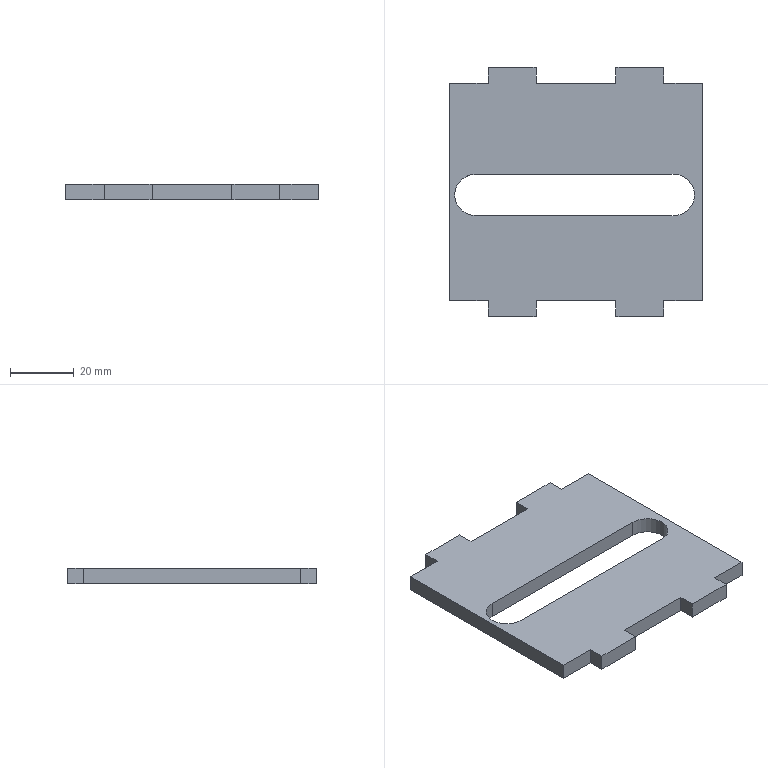Part | SolidWorks | features Extrusion 1, ICE 1 | 1 solid | 27 faces | box 79 x 77.9 x 5 mm | volume 23665 mm3 | plane 24 | cylinder 3 | commonest cylinder face diameters 12.879 x3
STEP:
#1=CARTESIAN_POINT('',(1.54,38.031,5.));
#2=VERTEX_POINT('',#1);
#3=CARTESIAN_POINT('',(7.98,44.471,5.));
#4=VERTEX_POINT('',#3);
#5=CARTESIAN_POINT('',(7.98,38.031,5.));
#6=DIRECTION('',(0.,0.,-1.));
#7=DIRECTION('',(-1.,0.,0.));
#8=AXIS2_PLACEMENT_3D('',#5,#6,#7);
#9=CIRCLE('',#8,6.44);
#10=EDGE_CURVE('',#2,#4,#9,.T.);
#11=ORIENTED_EDGE('',*,*,#10,.F.);
#12=CARTESIAN_POINT('',(1.54,38.031,0.));
#13=VERTEX_POINT('',#12);
#14=CARTESIAN_POINT('',(1.54,38.031,5.));
#15=DIRECTION('',(0.,0.,-1.));
#16=VECTOR('',#15,1000.);
#17=LINE('',#14,#16);
#18=EDGE_CURVE('',#2,#13,#17,.T.);
#19=ORIENTED_EDGE('',*,*,#18,.T.);
#20=CARTESIAN_POINT('',(7.98,44.471,0.));
#21=VERTEX_POINT('',#20);
#22=CARTESIAN_POINT('',(7.98,38.031,0.));
#23=DIRECTION('',(0.,0.,-1.));
#24=DIRECTION('',(-1.,0.,0.));
#25=AXIS2_PLACEMENT_3D('',#22,#23,#24);
#26=CIRCLE('',#25,6.44);
#27=EDGE_CURVE('',#13,#21,#26,.T.);
#28=ORIENTED_EDGE('',*,*,#27,.T.);
#29=CARTESIAN_POINT('',(7.98,44.471,5.));
#30=DIRECTION('',(0.,0.,-1.));
#31=VECTOR('',#30,1000.);
#32=LINE('',#29,#31);
#33=EDGE_CURVE('',#4,#21,#32,.T.);
#34=ORIENTED_EDGE('',*,*,#33,.F.);
#35=EDGE_LOOP('',(#11,#19,#28,#34));
#36=FACE_OUTER_BOUND('',#35,.T.);
#37=CARTESIAN_POINT('',(7.98,38.031,5.));
#38=DIRECTION('',(0.,0.,-1.));
#39=DIRECTION('',(-1.,0.,0.));
#40=AXIS2_PLACEMENT_3D('',#37,#38,#39);
#41=CYLINDRICAL_SURFACE('',#40,6.44);
#42=ADVANCED_FACE('',(#36),#41,.F.);
#43=CARTESIAN_POINT('',(52.,5.,0.));
#44=VERTEX_POINT('',#43);
#45=CARTESIAN_POINT('',(52.,0.,0.));
#46=VERTEX_POINT('',#45);
#47=CARTESIAN_POINT('',(52.,0.,0.));
#48=DIRECTION('',(0.,-1.,0.));
#49=VECTOR('',#48,1000.);
#50=LINE('',#47,#49);
#51=EDGE_CURVE('',#44,#46,#50,.T.);
#52=ORIENTED_EDGE('',*,*,#51,.T.);
#53=CARTESIAN_POINT('',(52.,0.,5.));
#54=VERTEX_POINT('',#53);
#55=CARTESIAN_POINT('',(52.,0.,5.));
#56=DIRECTION('',(0.,0.,-1.));
#57=VECTOR('',#56,1000.);
#58=LINE('',#55,#57);
#59=EDGE_CURVE('',#54,#46,#58,.T.);
#60=ORIENTED_EDGE('',*,*,#59,.F.);
#61=CARTESIAN_POINT('',(52.,5.,5.));
#62=VERTEX_POINT('',#61);
#63=CARTESIAN_POINT('',(52.,0.,5.));
#64=DIRECTION('',(0.,-1.,0.));
#65=VECTOR('',#64,1000.);
#66=LINE('',#63,#65);
#67=EDGE_CURVE('',#62,#54,#66,.T.);
#68=ORIENTED_EDGE('',*,*,#67,.F.);
#69=CARTESIAN_POINT('',(52.,5.,5.));
#70=DIRECTION('',(0.,0.,-1.));
#71=VECTOR('',#70,1000.);
#72=LINE('',#69,#71);
#73=EDGE_CURVE('',#62,#44,#72,.T.);
#74=ORIENTED_EDGE('',*,*,#73,.T.);
#75=EDGE_LOOP('',(#52,#60,#68,#74));
#76=FACE_OUTER_BOUND('',#75,.T.);
#77=CARTESIAN_POINT('',(52.,0.,5.));
#78=DIRECTION('',(1.,0.,0.));
#79=DIRECTION('',(0.,0.,-1.));
#80=AXIS2_PLACEMENT_3D('',#77,#78,#79);
#81=PLANE('',#80);
#82=ADVANCED_FACE('',(#76),#81,.F.);
#83=CARTESIAN_POINT('',(67.,0.,0.));
#84=VERTEX_POINT('',#83);
#85=CARTESIAN_POINT('',(52.,0.,0.));
#86=DIRECTION('',(1.,0.,0.));
#87=VECTOR('',#86,1000.);
#88=LINE('',#85,#87);
#89=EDGE_CURVE('',#46,#84,#88,.T.);
#90=ORIENTED_EDGE('',*,*,#89,.T.);
#91=CARTESIAN_POINT('',(67.,0.,5.));
#92=VERTEX_POINT('',#91);
#93=CARTESIAN_POINT('',(67.,0.,5.));
#94=DIRECTION('',(0.,0.,-1.));
#95=VECTOR('',#94,1000.);
#96=LINE('',#93,#95);
#97=EDGE_CURVE('',#92,#84,#96,.T.);
#98=ORIENTED_EDGE('',*,*,#97,.F.);
#99=CARTESIAN_POINT('',(52.,0.,5.));
#100=DIRECTION('',(1.,0.,0.));
#101=VECTOR('',#100,1000.);
#102=LINE('',#99,#101);
#103=EDGE_CURVE('',#54,#92,#102,.T.);
#104=ORIENTED_EDGE('',*,*,#103,.F.);
#105=ORIENTED_EDGE('',*,*,#59,.T.);
#106=EDGE_LOOP('',(#90,#98,#104,#105));
#107=FACE_OUTER_BOUND('',#106,.T.);
#108=CARTESIAN_POINT('',(52.,0.,5.));
#109=DIRECTION('',(0.,1.,0.));
#110=DIRECTION('',(-1.,0.,0.));
#111=AXIS2_PLACEMENT_3D('',#108,#109,#110);
#112=PLANE('',#111);
#113=ADVANCED_FACE('',(#107),#112,.F.);
#114=CARTESIAN_POINT('',(67.,5.,0.));
#115=VERTEX_POINT('',#114);
#116=CARTESIAN_POINT('',(67.,0.,0.));
#117=DIRECTION('',(0.,1.,0.));
#118=VECTOR('',#117,1000.);
#119=LINE('',#116,#118);
#120=EDGE_CURVE('',#84,#115,#119,.T.);
#121=ORIENTED_EDGE('',*,*,#120,.T.);
#122=CARTESIAN_POINT('',(67.,5.,5.));
#123=VERTEX_POINT('',#122);
#124=CARTESIAN_POINT('',(67.,5.,5.));
#125=DIRECTION('',(0.,0.,-1.));
#126=VECTOR('',#125,1000.);
#127=LINE('',#124,#126);
#128=EDGE_CURVE('',#123,#115,#127,.T.);
#129=ORIENTED_EDGE('',*,*,#128,.F.);
#130=CARTESIAN_POINT('',(67.,0.,5.));
#131=DIRECTION('',(0.,1.,0.));
#132=VECTOR('',#131,1000.);
#133=LINE('',#130,#132);
#134=EDGE_CURVE('',#92,#123,#133,.T.);
#135=ORIENTED_EDGE('',*,*,#134,.F.);
#136=ORIENTED_EDGE('',*,*,#97,.T.);
#137=EDGE_LOOP('',(#121,#129,#135,#136));
#138=FACE_OUTER_BOUND('',#137,.T.);
#139=CARTESIAN_POINT('',(67.,0.,5.));
#140=DIRECTION('',(-1.,0.,0.));
#141=DIRECTION('',(0.,0.,1.));
#142=AXIS2_PLACEMENT_3D('',#139,#140,#141);
#143=PLANE('',#142);
#144=ADVANCED_FACE('',(#138),#143,.F.);
#145=CARTESIAN_POINT('',(79.,5.,0.));
#146=VERTEX_POINT('',#145);
#147=CARTESIAN_POINT('',(67.,5.,0.));
#148=DIRECTION('',(1.,0.,0.));
#149=VECTOR('',#148,1000.);
#150=LINE('',#147,#149);
#151=EDGE_CURVE('',#115,#146,#150,.T.);
#152=ORIENTED_EDGE('',*,*,#151,.T.);
#153=CARTESIAN_POINT('',(79.,5.,5.));
#154=VERTEX_POINT('',#153);
#155=CARTESIAN_POINT('',(79.,5.,5.));
#156=DIRECTION('',(0.,0.,-1.));
#157=VECTOR('',#156,1000.);
#158=LINE('',#155,#157);
#159=EDGE_CURVE('',#154,#146,#158,.T.);
#160=ORIENTED_EDGE('',*,*,#159,.F.);
#161=CARTESIAN_POINT('',(67.,5.,5.));
#162=DIRECTION('',(1.,0.,0.));
#163=VECTOR('',#162,1000.);
#164=LINE('',#161,#163);
#165=EDGE_CURVE('',#123,#154,#164,.T.);
#166=ORIENTED_EDGE('',*,*,#165,.F.);
#167=ORIENTED_EDGE('',*,*,#128,.T.);
#168=EDGE_LOOP('',(#152,#160,#166,#167));
#169=FACE_OUTER_BOUND('',#168,.T.);
#170=CARTESIAN_POINT('',(67.,5.,5.));
#171=DIRECTION('',(0.,1.,0.));
#172=DIRECTION('',(-1.,0.,0.));
#173=AXIS2_PLACEMENT_3D('',#170,#171,#172);
#174=PLANE('',#173);
#175=ADVANCED_FACE('',(#169),#174,.F.);
#176=CARTESIAN_POINT('',(79.,72.9,0.));
#177=VERTEX_POINT('',#176);
#178=CARTESIAN_POINT('',(79.,5.,0.));
#179=DIRECTION('',(0.,1.,0.));
#180=VECTOR('',#179,1000.);
#181=LINE('',#178,#180);
#182=EDGE_CURVE('',#146,#177,#181,.T.);
#183=ORIENTED_EDGE('',*,*,#182,.T.);
#184=CARTESIAN_POINT('',(79.,72.9,5.));
#185=VERTEX_POINT('',#184);
#186=CARTESIAN_POINT('',(79.,72.9,5.));
#187=DIRECTION('',(0.,0.,-1.));
#188=VECTOR('',#187,1000.);
#189=LINE('',#186,#188);
#190=EDGE_CURVE('',#185,#177,#189,.T.);
#191=ORIENTED_EDGE('',*,*,#190,.F.);
#192=CARTESIAN_POINT('',(79.,5.,5.));
#193=DIRECTION('',(0.,1.,0.));
#194=VECTOR('',#193,1000.);
#195=LINE('',#192,#194);
#196=EDGE_CURVE('',#154,#185,#195,.T.);
#197=ORIENTED_EDGE('',*,*,#196,.F.);
#198=ORIENTED_EDGE('',*,*,#159,.T.);
#199=EDGE_LOOP('',(#183,#191,#197,#198));
#200=FACE_OUTER_BOUND('',#199,.T.);
#201=CARTESIAN_POINT('',(79.,5.,5.));
#202=DIRECTION('',(-1.,0.,0.));
#203=DIRECTION('',(0.,0.,1.));
#204=AXIS2_PLACEMENT_3D('',#201,#202,#203);
#205=PLANE('',#204);
#206=ADVANCED_FACE('',(#200),#205,.F.);
#207=CARTESIAN_POINT('',(67.,72.9,0.));
#208=VERTEX_POINT('',#207);
#209=CARTESIAN_POINT('',(79.,72.9,0.));
#210=DIRECTION('',(-1.,0.,0.));
#211=VECTOR('',#210,1000.);
#212=LINE('',#209,#211);
#213=EDGE_CURVE('',#177,#208,#212,.T.);
#214=ORIENTED_EDGE('',*,*,#213,.T.);
#215=CARTESIAN_POINT('',(67.,72.9,5.));
#216=VERTEX_POINT('',#215);
#217=CARTESIAN_POINT('',(67.,72.9,5.));
#218=DIRECTION('',(0.,0.,-1.));
#219=VECTOR('',#218,1000.);
#220=LINE('',#217,#219);
#221=EDGE_CURVE('',#216,#208,#220,.T.);
#222=ORIENTED_EDGE('',*,*,#221,.F.);
#223=CARTESIAN_POINT('',(79.,72.9,5.));
#224=DIRECTION('',(-1.,0.,0.));
#225=VECTOR('',#224,1000.);
#226=LINE('',#223,#225);
#227=EDGE_CURVE('',#185,#216,#226,.T.);
#228=ORIENTED_EDGE('',*,*,#227,.F.);
#229=ORIENTED_EDGE('',*,*,#190,.T.);
#230=EDGE_LOOP('',(#214,#222,#228,#229));
#231=FACE_OUTER_BOUND('',#230,.T.);
#232=CARTESIAN_POINT('',(79.,72.9,5.));
#233=DIRECTION('',(0.,-1.,0.));
#234=DIRECTION('',(0.,0.,-1.));
#235=AXIS2_PLACEMENT_3D('',#232,#233,#234);
#236=PLANE('',#235);
#237=ADVANCED_FACE('',(#231),#236,.F.);
#238=CARTESIAN_POINT('',(67.,77.9,0.));
#239=VERTEX_POINT('',#238);
#240=CARTESIAN_POINT('',(67.,77.9,0.));
#241=DIRECTION('',(0.,1.,0.));
#242=VECTOR('',#241,1000.);
#243=LINE('',#240,#242);
#244=EDGE_CURVE('',#208,#239,#243,.T.);
#245=ORIENTED_EDGE('',*,*,#244,.T.);
#246=CARTESIAN_POINT('',(67.,77.9,5.));
#247=VERTEX_POINT('',#246);
#248=CARTESIAN_POINT('',(67.,77.9,5.));
#249=DIRECTION('',(0.,0.,-1.));
#250=VECTOR('',#249,1000.);
#251=LINE('',#248,#250);
#252=EDGE_CURVE('',#247,#239,#251,.T.);
#253=ORIENTED_EDGE('',*,*,#252,.F.);
#254=CARTESIAN_POINT('',(67.,77.9,5.));
#255=DIRECTION('',(0.,1.,0.));
#256=VECTOR('',#255,1000.);
#257=LINE('',#254,#256);
#258=EDGE_CURVE('',#216,#247,#257,.T.);
#259=ORIENTED_EDGE('',*,*,#258,.F.);
#260=ORIENTED_EDGE('',*,*,#221,.T.);
#261=EDGE_LOOP('',(#245,#253,#259,#260));
#262=FACE_OUTER_BOUND('',#261,.T.);
#263=CARTESIAN_POINT('',(67.,77.9,5.));
#264=DIRECTION('',(-1.,0.,0.));
#265=DIRECTION('',(0.,0.,1.));
#266=AXIS2_PLACEMENT_3D('',#263,#264,#265);
#267=PLANE('',#266);
#268=ADVANCED_FACE('',(#262),#267,.F.);
#269=CARTESIAN_POINT('',(52.,77.9,0.));
#270=VERTEX_POINT('',#269);
#271=CARTESIAN_POINT('',(52.,77.9,0.));
#272=DIRECTION('',(-1.,0.,0.));
#273=VECTOR('',#272,1000.);
#274=LINE('',#271,#273);
#275=EDGE_CURVE('',#239,#270,#274,.T.);
#276=ORIENTED_EDGE('',*,*,#275,.T.);
#277=CARTESIAN_POINT('',(52.,77.9,5.));
#278=VERTEX_POINT('',#277);
#279=CARTESIAN_POINT('',(52.,77.9,5.));
#280=DIRECTION('',(0.,0.,-1.));
#281=VECTOR('',#280,1000.);
#282=LINE('',#279,#281);
#283=EDGE_CURVE('',#278,#270,#282,.T.);
#284=ORIENTED_EDGE('',*,*,#283,.F.);
#285=CARTESIAN_POINT('',(52.,77.9,5.));
#286=DIRECTION('',(-1.,0.,0.));
#287=VECTOR('',#286,1000.);
#288=LINE('',#285,#287);
#289=EDGE_CURVE('',#247,#278,#288,.T.);
#290=ORIENTED_EDGE('',*,*,#289,.F.);
#291=ORIENTED_EDGE('',*,*,#252,.T.);
#292=EDGE_LOOP('',(#276,#284,#290,#291));
#293=FACE_OUTER_BOUND('',#292,.T.);
#294=CARTESIAN_POINT('',(52.,77.9,5.));
#295=DIRECTION('',(0.,-1.,0.));
#296=DIRECTION('',(0.,0.,-1.));
#297=AXIS2_PLACEMENT_3D('',#294,#295,#296);
#298=PLANE('',#297);
#299=ADVANCED_FACE('',(#293),#298,.F.);
#300=CARTESIAN_POINT('',(52.,72.9,0.));
#301=VERTEX_POINT('',#300);
#302=CARTESIAN_POINT('',(52.,77.9,0.));
#303=DIRECTION('',(0.,-1.,0.));
#304=VECTOR('',#303,1000.);
#305=LINE('',#302,#304);
#306=EDGE_CURVE('',#270,#301,#305,.T.);
#307=ORIENTED_EDGE('',*,*,#306,.T.);
#308=CARTESIAN_POINT('',(52.,72.9,5.));
#309=VERTEX_POINT('',#308);
#310=CARTESIAN_POINT('',(52.,72.9,5.));
#311=DIRECTION('',(0.,0.,-1.));
#312=VECTOR('',#311,1000.);
#313=LINE('',#310,#312);
#314=EDGE_CURVE('',#309,#301,#313,.T.);
#315=ORIENTED_EDGE('',*,*,#314,.F.);
#316=CARTESIAN_POINT('',(52.,77.9,5.));
#317=DIRECTION('',(0.,-1.,0.));
#318=VECTOR('',#317,1000.);
#319=LINE('',#316,#318);
#320=EDGE_CURVE('',#278,#309,#319,.T.);
#321=ORIENTED_EDGE('',*,*,#320,.F.);
#322=ORIENTED_EDGE('',*,*,#283,.T.);
#323=EDGE_LOOP('',(#307,#315,#321,#322));
#324=FACE_OUTER_BOUND('',#323,.T.);
#325=CARTESIAN_POINT('',(52.,77.9,5.));
#326=DIRECTION('',(1.,0.,0.));
#327=DIRECTION('',(0.,1.,0.));
#328=AXIS2_PLACEMENT_3D('',#325,#326,#327);
#329=PLANE('',#328);
#330=ADVANCED_FACE('',(#324),#329,.F.);
#331=CARTESIAN_POINT('',(27.,72.9,0.));
#332=VERTEX_POINT('',#331);
#333=CARTESIAN_POINT('',(52.,72.9,0.));
#334=DIRECTION('',(-1.,0.,0.));
#335=VECTOR('',#334,1000.);
#336=LINE('',#333,#335);
#337=EDGE_CURVE('',#301,#332,#336,.T.);
#338=ORIENTED_EDGE('',*,*,#337,.T.);
#339=CARTESIAN_POINT('',(27.,72.9,5.));
#340=VERTEX_POINT('',#339);
#341=CARTESIAN_POINT('',(27.,72.9,5.));
#342=DIRECTION('',(0.,0.,-1.));
#343=VECTOR('',#342,1000.);
#344=LINE('',#341,#343);
#345=EDGE_CURVE('',#340,#332,#344,.T.);
#346=ORIENTED_EDGE('',*,*,#345,.F.);
#347=CARTESIAN_POINT('',(52.,72.9,5.));
#348=DIRECTION('',(-1.,0.,0.));
#349=VECTOR('',#348,1000.);
#350=LINE('',#347,#349);
#351=EDGE_CURVE('',#309,#340,#350,.T.);
#352=ORIENTED_EDGE('',*,*,#351,.F.);
#353=ORIENTED_EDGE('',*,*,#314,.T.);
#354=EDGE_LOOP('',(#338,#346,#352,#353));
#355=FACE_OUTER_BOUND('',#354,.T.);
#356=CARTESIAN_POINT('',(52.,72.9,5.));
#357=DIRECTION('',(0.,-1.,0.));
#358=DIRECTION('',(0.,0.,-1.));
#359=AXIS2_PLACEMENT_3D('',#356,#357,#358);
#360=PLANE('',#359);
#361=ADVANCED_FACE('',(#355),#360,.F.);
#362=CARTESIAN_POINT('',(27.,77.9,0.));
#363=VERTEX_POINT('',#362);
#364=CARTESIAN_POINT('',(27.,77.9,0.));
#365=DIRECTION('',(0.,1.,0.));
#366=VECTOR('',#365,1000.);
#367=LINE('',#364,#366);
#368=EDGE_CURVE('',#332,#363,#367,.T.);
#369=ORIENTED_EDGE('',*,*,#368,.T.);
#370=CARTESIAN_POINT('',(27.,77.9,5.));
#371=VERTEX_POINT('',#370);
#372=CARTESIAN_POINT('',(27.,77.9,5.));
#373=DIRECTION('',(0.,0.,-1.));
#374=VECTOR('',#373,1000.);
#375=LINE('',#372,#374);
#376=EDGE_CURVE('',#371,#363,#375,.T.);
#377=ORIENTED_EDGE('',*,*,#376,.F.);
#378=CARTESIAN_POINT('',(27.,77.9,5.));
#379=DIRECTION('',(0.,1.,0.));
#380=VECTOR('',#379,1000.);
#381=LINE('',#378,#380);
#382=EDGE_CURVE('',#340,#371,#381,.T.);
#383=ORIENTED_EDGE('',*,*,#382,.F.);
#384=ORIENTED_EDGE('',*,*,#345,.T.);
#385=EDGE_LOOP('',(#369,#377,#383,#384));
#386=FACE_OUTER_BOUND('',#385,.T.);
#387=CARTESIAN_POINT('',(27.,77.9,5.));
#388=DIRECTION('',(-1.,0.,0.));
#389=DIRECTION('',(0.,-1.,0.));
#390=AXIS2_PLACEMENT_3D('',#387,#388,#389);
#391=PLANE('',#390);
#392=ADVANCED_FACE('',(#386),#391,.F.);
#393=CARTESIAN_POINT('',(12.,77.9,0.));
#394=VERTEX_POINT('',#393);
#395=CARTESIAN_POINT('',(12.,77.9,0.));
#396=DIRECTION('',(-1.,0.,0.));
#397=VECTOR('',#396,1000.);
#398=LINE('',#395,#397);
#399=EDGE_CURVE('',#363,#394,#398,.T.);
#400=ORIENTED_EDGE('',*,*,#399,.T.);
#401=CARTESIAN_POINT('',(12.,77.9,5.));
#402=VERTEX_POINT('',#401);
#403=CARTESIAN_POINT('',(12.,77.9,5.));
#404=DIRECTION('',(0.,0.,-1.));
#405=VECTOR('',#404,1000.);
#406=LINE('',#403,#405);
#407=EDGE_CURVE('',#402,#394,#406,.T.);
#408=ORIENTED_EDGE('',*,*,#407,.F.);
#409=CARTESIAN_POINT('',(12.,77.9,5.));
#410=DIRECTION('',(-1.,0.,0.));
#411=VECTOR('',#410,1000.);
#412=LINE('',#409,#411);
#413=EDGE_CURVE('',#371,#402,#412,.T.);
#414=ORIENTED_EDGE('',*,*,#413,.F.);
#415=ORIENTED_EDGE('',*,*,#376,.T.);
#416=EDGE_LOOP('',(#400,#408,#414,#415));
#417=FACE_OUTER_BOUND('',#416,.T.);
#418=CARTESIAN_POINT('',(12.,77.9,5.));
#419=DIRECTION('',(0.,-1.,0.));
#420=DIRECTION('',(0.,0.,-1.));
#421=AXIS2_PLACEMENT_3D('',#418,#419,#420);
#422=PLANE('',#421);
#423=ADVANCED_FACE('',(#417),#422,.F.);
#424=CARTESIAN_POINT('',(12.,72.9,0.));
#425=VERTEX_POINT('',#424);
#426=CARTESIAN_POINT('',(12.,77.9,0.));
#427=DIRECTION('',(0.,-1.,0.));
#428=VECTOR('',#427,1000.);
#429=LINE('',#426,#428);
#430=EDGE_CURVE('',#394,#425,#429,.T.);
#431=ORIENTED_EDGE('',*,*,#430,.T.);
#432=CARTESIAN_POINT('',(12.,72.9,5.));
#433=VERTEX_POINT('',#432);
#434=CARTESIAN_POINT('',(12.,72.9,5.));
#435=DIRECTION('',(0.,0.,-1.));
#436=VECTOR('',#435,1000.);
#437=LINE('',#434,#436);
#438=EDGE_CURVE('',#433,#425,#437,.T.);
#439=ORIENTED_EDGE('',*,*,#438,.F.);
#440=CARTESIAN_POINT('',(12.,77.9,5.));
#441=DIRECTION('',(0.,-1.,0.));
#442=VECTOR('',#441,1000.);
#443=LINE('',#440,#442);
#444=EDGE_CURVE('',#402,#433,#443,.T.);
#445=ORIENTED_EDGE('',*,*,#444,.F.);
#446=ORIENTED_EDGE('',*,*,#407,.T.);
#447=EDGE_LOOP('',(#431,#439,#445,#446));
#448=FACE_OUTER_BOUND('',#447,.T.);
#449=CARTESIAN_POINT('',(12.,77.9,5.));
#450=DIRECTION('',(1.,0.,0.));
#451=DIRECTION('',(0.,0.,-1.));
#452=AXIS2_PLACEMENT_3D('',#449,#450,#451);
#453=PLANE('',#452);
#454=ADVANCED_FACE('',(#448),#453,.F.);
#455=CARTESIAN_POINT('',(0.,72.9,0.));
#456=VERTEX_POINT('',#455);
#457=CARTESIAN_POINT('',(12.,72.9,0.));
#458=DIRECTION('',(-1.,0.,0.));
#459=VECTOR('',#458,1000.);
#460=LINE('',#457,#459);
#461=EDGE_CURVE('',#425,#456,#460,.T.);
#462=ORIENTED_EDGE('',*,*,#461,.T.);
#463=CARTESIAN_POINT('',(0.,72.9,5.));
#464=VERTEX_POINT('',#463);
#465=CARTESIAN_POINT('',(0.,72.9,5.));
#466=DIRECTION('',(0.,0.,-1.));
#467=VECTOR('',#466,1000.);
#468=LINE('',#465,#467);
#469=EDGE_CURVE('',#464,#456,#468,.T.);
#470=ORIENTED_EDGE('',*,*,#469,.F.);
#471=CARTESIAN_POINT('',(12.,72.9,5.));
#472=DIRECTION('',(-1.,0.,0.));
#473=VECTOR('',#472,1000.);
#474=LINE('',#471,#473);
#475=EDGE_CURVE('',#433,#464,#474,.T.);
#476=ORIENTED_EDGE('',*,*,#475,.F.);
#477=ORIENTED_EDGE('',*,*,#438,.T.);
#478=EDGE_LOOP('',(#462,#470,#476,#477));
#479=FACE_OUTER_BOUND('',#478,.T.);
#480=CARTESIAN_POINT('',(12.,72.9,5.));
#481=DIRECTION('',(0.,-1.,0.));
#482=DIRECTION('',(0.,0.,-1.));
#483=AXIS2_PLACEMENT_3D('',#480,#481,#482);
#484=PLANE('',#483);
#485=ADVANCED_FACE('',(#479),#484,.F.);
#486=CARTESIAN_POINT('',(0.,5.,0.));
#487=VERTEX_POINT('',#486);
#488=CARTESIAN_POINT('',(0.,5.,0.));
#489=DIRECTION('',(0.,-1.,0.));
#490=VECTOR('',#489,1000.);
#491=LINE('',#488,#490);
#492=EDGE_CURVE('',#456,#487,#491,.T.);
#493=ORIENTED_EDGE('',*,*,#492,.T.);
#494=CARTESIAN_POINT('',(0.,5.,5.));
#495=VERTEX_POINT('',#494);
#496=CARTESIAN_POINT('',(0.,5.,5.));
#497=DIRECTION('',(0.,0.,-1.));
#498=VECTOR('',#497,1000.);
#499=LINE('',#496,#498);
#500=EDGE_CURVE('',#495,#487,#499,.T.);
#501=ORIENTED_EDGE('',*,*,#500,.F.);
#502=CARTESIAN_POINT('',(0.,5.,5.));
#503=DIRECTION('',(0.,-1.,0.));
#504=VECTOR('',#503,1000.);
#505=LINE('',#502,#504);
#506=EDGE_CURVE('',#464,#495,#505,.T.);
#507=ORIENTED_EDGE('',*,*,#506,.F.);
#508=ORIENTED_EDGE('',*,*,#469,.T.);
#509=EDGE_LOOP('',(#493,#501,#507,#508));
#510=FACE_OUTER_BOUND('',#509,.T.);
#511=CARTESIAN_POINT('',(0.,5.,5.));
#512=DIRECTION('',(1.,0.,0.));
#513=DIRECTION('',(0.,1.,0.));
#514=AXIS2_PLACEMENT_3D('',#511,#512,#513);
#515=PLANE('',#514);
#516=ADVANCED_FACE('',(#510),#515,.F.);
#517=CARTESIAN_POINT('',(12.,5.,0.));
#518=VERTEX_POINT('',#517);
#519=CARTESIAN_POINT('',(0.,5.,0.));
#520=DIRECTION('',(1.,0.,0.));
#521=VECTOR('',#520,1000.);
#522=LINE('',#519,#521);
#523=EDGE_CURVE('',#487,#518,#522,.T.);
#524=ORIENTED_EDGE('',*,*,#523,.T.);
#525=CARTESIAN_POINT('',(12.,5.,5.));
#526=VERTEX_POINT('',#525);
#527=CARTESIAN_POINT('',(12.,5.,5.));
#528=DIRECTION('',(0.,0.,-1.));
#529=VECTOR('',#528,1000.);
#530=LINE('',#527,#529);
#531=EDGE_CURVE('',#526,#518,#530,.T.);
#532=ORIENTED_EDGE('',*,*,#531,.F.);
#533=CARTESIAN_POINT('',(0.,5.,5.));
#534=DIRECTION('',(1.,0.,0.));
#535=VECTOR('',#534,1000.);
#536=LINE('',#533,#535);
#537=EDGE_CURVE('',#495,#526,#536,.T.);
#538=ORIENTED_EDGE('',*,*,#537,.F.);
#539=ORIENTED_EDGE('',*,*,#500,.T.);
#540=EDGE_LOOP('',(#524,#532,#538,#539));
#541=FACE_OUTER_BOUND('',#540,.T.);
#542=CARTESIAN_POINT('',(0.,5.,5.));
#543=DIRECTION('',(0.,1.,0.));
#544=DIRECTION('',(-1.,0.,0.));
#545=AXIS2_PLACEMENT_3D('',#542,#543,#544);
#546=PLANE('',#545);
#547=ADVANCED_FACE('',(#541),#546,.F.);
#548=CARTESIAN_POINT('',(12.,0.,0.));
#549=VERTEX_POINT('',#548);
#550=CARTESIAN_POINT('',(12.,0.,0.));
#551=DIRECTION('',(0.,-1.,0.));
#552=VECTOR('',#551,1000.);
#553=LINE('',#550,#552);
#554=EDGE_CURVE('',#518,#549,#553,.T.);
#555=ORIENTED_EDGE('',*,*,#554,.T.);
#556=CARTESIAN_POINT('',(12.,0.,5.));
#557=VERTEX_POINT('',#556);
#558=CARTESIAN_POINT('',(12.,0.,5.));
#559=DIRECTION('',(0.,0.,-1.));
#560=VECTOR('',#559,1000.);
#561=LINE('',#558,#560);
#562=EDGE_CURVE('',#557,#549,#561,.T.);
#563=ORIENTED_EDGE('',*,*,#562,.F.);
#564=CARTESIAN_POINT('',(12.,0.,5.));
#565=DIRECTION('',(0.,-1.,0.));
#566=VECTOR('',#565,1000.);
#567=LINE('',#564,#566);
#568=EDGE_CURVE('',#526,#557,#567,.T.);
#569=ORIENTED_EDGE('',*,*,#568,.F.);
#570=ORIENTED_EDGE('',*,*,#531,.T.);
#571=EDGE_LOOP('',(#555,#563,#569,#570));
#572=FACE_OUTER_BOUND('',#571,.T.);
#573=CARTESIAN_POINT('',(12.,0.,5.));
#574=DIRECTION('',(1.,0.,0.));
#575=DIRECTION('',(0.,0.,-1.));
#576=AXIS2_PLACEMENT_3D('',#573,#574,#575);
#577=PLANE('',#576);
#578=ADVANCED_FACE('',(#572),#577,.F.);
#579=CARTESIAN_POINT('',(27.,0.,0.));
#580=VERTEX_POINT('',#579);
#581=CARTESIAN_POINT('',(12.,0.,0.));
#582=DIRECTION('',(1.,0.,0.));
#583=VECTOR('',#582,1000.);
#584=LINE('',#581,#583);
#585=EDGE_CURVE('',#549,#580,#584,.T.);
#586=ORIENTED_EDGE('',*,*,#585,.T.);
#587=CARTESIAN_POINT('',(27.,0.,5.));
#588=VERTEX_POINT('',#587);
#589=CARTESIAN_POINT('',(27.,0.,5.));
#590=DIRECTION('',(0.,0.,-1.));
#591=VECTOR('',#590,1000.);
#592=LINE('',#589,#591);
#593=EDGE_CURVE('',#588,#580,#592,.T.);
#594=ORIENTED_EDGE('',*,*,#593,.F.);
#595=CARTESIAN_POINT('',(12.,0.,5.));
#596=DIRECTION('',(1.,0.,0.));
#597=VECTOR('',#596,1000.);
#598=LINE('',#595,#597);
#599=EDGE_CURVE('',#557,#588,#598,.T.);
#600=ORIENTED_EDGE('',*,*,#599,.F.);
#601=ORIENTED_EDGE('',*,*,#562,.T.);
#602=EDGE_LOOP('',(#586,#594,#600,#601));
#603=FACE_OUTER_BOUND('',#602,.T.);
#604=CARTESIAN_POINT('',(12.,0.,5.));
#605=DIRECTION('',(0.,1.,0.));
#606=DIRECTION('',(-1.,0.,0.));
#607=AXIS2_PLACEMENT_3D('',#604,#605,#606);
#608=PLANE('',#607);
#609=ADVANCED_FACE('',(#603),#608,.F.);
#610=CARTESIAN_POINT('',(27.,5.,0.));
#611=VERTEX_POINT('',#610);
#612=CARTESIAN_POINT('',(27.,0.,0.));
#613=DIRECTION('',(0.,1.,0.));
#614=VECTOR('',#613,1000.);
#615=LINE('',#612,#614);
#616=EDGE_CURVE('',#580,#611,#615,.T.);
#617=ORIENTED_EDGE('',*,*,#616,.T.);
#618=CARTESIAN_POINT('',(27.,5.,5.));
#619=VERTEX_POINT('',#618);
#620=CARTESIAN_POINT('',(27.,5.,5.));
#621=DIRECTION('',(0.,0.,-1.));
#622=VECTOR('',#621,1000.);
#623=LINE('',#620,#622);
#624=EDGE_CURVE('',#619,#611,#623,.T.);
#625=ORIENTED_EDGE('',*,*,#624,.F.);
#626=CARTESIAN_POINT('',(27.,0.,5.));
#627=DIRECTION('',(0.,1.,0.));
#628=VECTOR('',#627,1000.);
#629=LINE('',#626,#628);
#630=EDGE_CURVE('',#588,#619,#629,.T.);
#631=ORIENTED_EDGE('',*,*,#630,.F.);
#632=ORIENTED_EDGE('',*,*,#593,.T.);
#633=EDGE_LOOP('',(#617,#625,#631,#632));
#634=FACE_OUTER_BOUND('',#633,.T.);
#635=CARTESIAN_POINT('',(27.,0.,5.));
#636=DIRECTION('',(-1.,0.,0.));
#637=DIRECTION('',(0.,0.,1.));
#638=AXIS2_PLACEMENT_3D('',#635,#636,#637);
#639=PLANE('',#638);
#640=ADVANCED_FACE('',(#634),#639,.F.);
#641=CARTESIAN_POINT('',(27.,5.,0.));
#642=DIRECTION('',(1.,0.,0.));
#643=VECTOR('',#642,1000.);
#644=LINE('',#641,#643);
#645=EDGE_CURVE('',#611,#44,#644,.T.);
#646=ORIENTED_EDGE('',*,*,#645,.T.);
#647=ORIENTED_EDGE('',*,*,#73,.F.);
#648=CARTESIAN_POINT('',(27.,5.,5.));
#649=DIRECTION('',(1.,0.,0.));
#650=VECTOR('',#649,1000.);
#651=LINE('',#648,#650);
#652=EDGE_CURVE('',#619,#62,#651,.T.);
#653=ORIENTED_EDGE('',*,*,#652,.F.);
#654=ORIENTED_EDGE('',*,*,#624,.T.);
#655=EDGE_LOOP('',(#646,#647,#653,#654));
#656=FACE_OUTER_BOUND('',#655,.T.);
#657=CARTESIAN_POINT('',(27.,5.,5.));
#658=DIRECTION('',(0.,1.,0.));
#659=DIRECTION('',(0.,0.,1.));
#660=AXIS2_PLACEMENT_3D('',#657,#658,#659);
#661=PLANE('',#660);
#662=ADVANCED_FACE('',(#656),#661,.F.);
#663=CARTESIAN_POINT('',(70.163,44.471,5.));
#664=VERTEX_POINT('',#663);
#665=CARTESIAN_POINT('',(70.163,44.471,5.));
#666=DIRECTION('',(1.,0.,0.));
#667=VECTOR('',#666,1000.);
#668=LINE('',#665,#667);
#669=EDGE_CURVE('',#4,#664,#668,.T.);
#670=ORIENTED_EDGE('',*,*,#669,.T.);
#671=CARTESIAN_POINT('',(70.163,31.592,5.));
#672=VERTEX_POINT('',#671);
#673=CARTESIAN_POINT('',(70.163,38.031,5.));
#674=DIRECTION('',(0.,0.,-1.));
#675=DIRECTION('',(-1.,0.,0.));
#676=AXIS2_PLACEMENT_3D('',#673,#674,#675);
#677=CIRCLE('',#676,6.44);
#678=EDGE_CURVE('',#664,#672,#677,.T.);
#679=ORIENTED_EDGE('',*,*,#678,.T.);
#680=CARTESIAN_POINT('',(7.98,31.592,5.));
#681=VERTEX_POINT('',#680);
#682=CARTESIAN_POINT('',(70.163,31.592,5.));
#683=DIRECTION('',(-1.,0.,0.));
#684=VECTOR('',#683,1000.);
#685=LINE('',#682,#684);
#686=EDGE_CURVE('',#672,#681,#685,.T.);
#687=ORIENTED_EDGE('',*,*,#686,.T.);
#688=CARTESIAN_POINT('',(7.98,38.031,5.));
#689=DIRECTION('',(0.,0.,-1.));
#690=DIRECTION('',(-1.,0.,0.));
#691=AXIS2_PLACEMENT_3D('',#688,#689,#690);
#692=CIRCLE('',#691,6.44);
#693=EDGE_CURVE('',#681,#2,#692,.T.);
#694=ORIENTED_EDGE('',*,*,#693,.T.);
#695=ORIENTED_EDGE('',*,*,#10,.T.);
#696=EDGE_LOOP('',(#670,#679,#687,#694,#695));
#697=FACE_BOUND('',#696,.T.);
#698=ORIENTED_EDGE('',*,*,#67,.T.);
#699=ORIENTED_EDGE('',*,*,#103,.T.);
#700=ORIENTED_EDGE('',*,*,#134,.T.);
#701=ORIENTED_EDGE('',*,*,#165,.T.);
#702=ORIENTED_EDGE('',*,*,#196,.T.);
#703=ORIENTED_EDGE('',*,*,#227,.T.);
#704=ORIENTED_EDGE('',*,*,#258,.T.);
#705=ORIENTED_EDGE('',*,*,#289,.T.);
#706=ORIENTED_EDGE('',*,*,#320,.T.);
#707=ORIENTED_EDGE('',*,*,#351,.T.);
#708=ORIENTED_EDGE('',*,*,#382,.T.);
#709=ORIENTED_EDGE('',*,*,#413,.T.);
#710=ORIENTED_EDGE('',*,*,#444,.T.);
#711=ORIENTED_EDGE('',*,*,#475,.T.);
#712=ORIENTED_EDGE('',*,*,#506,.T.);
#713=ORIENTED_EDGE('',*,*,#537,.T.);
#714=ORIENTED_EDGE('',*,*,#568,.T.);
#715=ORIENTED_EDGE('',*,*,#599,.T.);
#716=ORIENTED_EDGE('',*,*,#630,.T.);
#717=ORIENTED_EDGE('',*,*,#652,.T.);
#718=EDGE_LOOP('',(#698,#699,#700,#701,#702,#703,#704,#705,#706,#707,#708,#709,#710,#711,#712,#713,#714,#715,#716,#717));
#719=FACE_OUTER_BOUND('',#718,.T.);
#720=CARTESIAN_POINT('',(0.,0.,5.));
#721=DIRECTION('',(0.,0.,-1.));
#722=DIRECTION('',(-1.,0.,0.));
#723=AXIS2_PLACEMENT_3D('',#720,#721,#722);
#724=PLANE('',#723);
#725=ADVANCED_FACE('',(#697,#719),#724,.F.);
#726=CARTESIAN_POINT('',(70.163,44.471,0.));
#727=VERTEX_POINT('',#726);
#728=CARTESIAN_POINT('',(70.163,31.592,0.));
#729=VERTEX_POINT('',#728);
#730=CARTESIAN_POINT('',(70.163,38.031,0.));
#731=DIRECTION('',(0.,0.,-1.));
#732=DIRECTION('',(-1.,0.,0.));
#733=AXIS2_PLACEMENT_3D('',#730,#731,#732);
#734=CIRCLE('',#733,6.44);
#735=EDGE_CURVE('',#727,#729,#734,.T.);
#736=ORIENTED_EDGE('',*,*,#735,.F.);
#737=CARTESIAN_POINT('',(70.163,44.471,0.));
#738=DIRECTION('',(1.,0.,0.));
#739=VECTOR('',#738,1000.);
#740=LINE('',#737,#739);
#741=EDGE_CURVE('',#21,#727,#740,.T.);
#742=ORIENTED_EDGE('',*,*,#741,.F.);
#743=ORIENTED_EDGE('',*,*,#27,.F.);
#744=CARTESIAN_POINT('',(7.98,31.592,0.));
#745=VERTEX_POINT('',#744);
#746=CARTESIAN_POINT('',(7.98,38.031,0.));
#747=DIRECTION('',(0.,0.,-1.));
#748=DIRECTION('',(-1.,0.,0.));
#749=AXIS2_PLACEMENT_3D('',#746,#747,#748);
#750=CIRCLE('',#749,6.44);
#751=EDGE_CURVE('',#745,#13,#750,.T.);
#752=ORIENTED_EDGE('',*,*,#751,.F.);
#753=CARTESIAN_POINT('',(70.163,31.592,0.));
#754=DIRECTION('',(-1.,0.,0.));
#755=VECTOR('',#754,1000.);
#756=LINE('',#753,#755);
#757=EDGE_CURVE('',#729,#745,#756,.T.);
#758=ORIENTED_EDGE('',*,*,#757,.F.);
#759=EDGE_LOOP('',(#736,#742,#743,#752,#758));
#760=FACE_BOUND('',#759,.T.);
#761=ORIENTED_EDGE('',*,*,#51,.F.);
#762=ORIENTED_EDGE('',*,*,#645,.F.);
#763=ORIENTED_EDGE('',*,*,#616,.F.);
#764=ORIENTED_EDGE('',*,*,#585,.F.);
#765=ORIENTED_EDGE('',*,*,#554,.F.);
#766=ORIENTED_EDGE('',*,*,#523,.F.);
#767=ORIENTED_EDGE('',*,*,#492,.F.);
#768=ORIENTED_EDGE('',*,*,#461,.F.);
#769=ORIENTED_EDGE('',*,*,#430,.F.);
#770=ORIENTED_EDGE('',*,*,#399,.F.);
#771=ORIENTED_EDGE('',*,*,#368,.F.);
#772=ORIENTED_EDGE('',*,*,#337,.F.);
#773=ORIENTED_EDGE('',*,*,#306,.F.);
#774=ORIENTED_EDGE('',*,*,#275,.F.);
#775=ORIENTED_EDGE('',*,*,#244,.F.);
#776=ORIENTED_EDGE('',*,*,#213,.F.);
#777=ORIENTED_EDGE('',*,*,#182,.F.);
#778=ORIENTED_EDGE('',*,*,#151,.F.);
#779=ORIENTED_EDGE('',*,*,#120,.F.);
#780=ORIENTED_EDGE('',*,*,#89,.F.);
#781=EDGE_LOOP('',(#761,#762,#763,#764,#765,#766,#767,#768,#769,#770,#771,#772,#773,#774,#775,#776,#777,#778,#779,#780));
#782=FACE_OUTER_BOUND('',#781,.T.);
#783=CARTESIAN_POINT('',(0.,0.,0.));
#784=DIRECTION('',(0.,0.,-1.));
#785=DIRECTION('',(-1.,0.,0.));
#786=AXIS2_PLACEMENT_3D('',#783,#784,#785);
#787=PLANE('',#786);
#788=ADVANCED_FACE('',(#760,#782),#787,.T.);
#789=ORIENTED_EDGE('',*,*,#735,.T.);
#790=CARTESIAN_POINT('',(70.163,31.592,5.));
#791=DIRECTION('',(0.,0.,-1.));
#792=VECTOR('',#791,1000.);
#793=LINE('',#790,#792);
#794=EDGE_CURVE('',#672,#729,#793,.T.);
#795=ORIENTED_EDGE('',*,*,#794,.F.);
#796=ORIENTED_EDGE('',*,*,#678,.F.);
#797=CARTESIAN_POINT('',(70.163,44.471,5.));
#798=DIRECTION('',(0.,0.,-1.));
#799=VECTOR('',#798,1000.);
#800=LINE('',#797,#799);
#801=EDGE_CURVE('',#664,#727,#800,.T.);
#802=ORIENTED_EDGE('',*,*,#801,.T.);
#803=EDGE_LOOP('',(#789,#795,#796,#802));
#804=FACE_OUTER_BOUND('',#803,.T.);
#805=CARTESIAN_POINT('',(70.163,38.031,5.));
#806=DIRECTION('',(0.,0.,-1.));
#807=DIRECTION('',(-1.,0.,0.));
#808=AXIS2_PLACEMENT_3D('',#805,#806,#807);
#809=CYLINDRICAL_SURFACE('',#808,6.44);
#810=ADVANCED_FACE('',(#804),#809,.F.);
#811=ORIENTED_EDGE('',*,*,#741,.T.);
#812=ORIENTED_EDGE('',*,*,#801,.F.);
#813=ORIENTED_EDGE('',*,*,#669,.F.);
#814=ORIENTED_EDGE('',*,*,#33,.T.);
#815=EDGE_LOOP('',(#811,#812,#813,#814));
#816=FACE_OUTER_BOUND('',#815,.T.);
#817=CARTESIAN_POINT('',(70.163,44.471,5.));
#818=DIRECTION('',(0.,1.,0.));
#819=DIRECTION('',(0.,0.,1.));
#820=AXIS2_PLACEMENT_3D('',#817,#818,#819);
#821=PLANE('',#820);
#822=ADVANCED_FACE('',(#816),#821,.F.);
#823=ORIENTED_EDGE('',*,*,#18,.F.);
#824=ORIENTED_EDGE('',*,*,#693,.F.);
#825=CARTESIAN_POINT('',(7.98,31.592,5.));
#826=DIRECTION('',(0.,0.,-1.));
#827=VECTOR('',#826,1000.);
#828=LINE('',#825,#827);
#829=EDGE_CURVE('',#681,#745,#828,.T.);
#830=ORIENTED_EDGE('',*,*,#829,.T.);
#831=ORIENTED_EDGE('',*,*,#751,.T.);
#832=EDGE_LOOP('',(#823,#824,#830,#831));
#833=FACE_OUTER_BOUND('',#832,.T.);
#834=CARTESIAN_POINT('',(7.98,38.031,5.));
#835=DIRECTION('',(0.,0.,-1.));
#836=DIRECTION('',(-1.,0.,0.));
#837=AXIS2_PLACEMENT_3D('',#834,#835,#836);
#838=CYLINDRICAL_SURFACE('',#837,6.44);
#839=ADVANCED_FACE('',(#833),#838,.F.);
#840=ORIENTED_EDGE('',*,*,#757,.T.);
#841=ORIENTED_EDGE('',*,*,#829,.F.);
#842=ORIENTED_EDGE('',*,*,#686,.F.);
#843=ORIENTED_EDGE('',*,*,#794,.T.);
#844=EDGE_LOOP('',(#840,#841,#842,#843));
#845=FACE_OUTER_BOUND('',#844,.T.);
#846=CARTESIAN_POINT('',(70.163,31.592,5.));
#847=DIRECTION('',(0.,-1.,0.));
#848=DIRECTION('',(0.,0.,-1.));
#849=AXIS2_PLACEMENT_3D('',#846,#847,#848);
#850=PLANE('',#849);
#851=ADVANCED_FACE('',(#845),#850,.F.);
#852=CLOSED_SHELL('',(#42,#82,#113,#144,#175,#206,#237,#268,#299,#330,#361,#392,#423,#454,#485,#516,#547,#578,#609,#640,#662,#725,#788,#810,#822,#839,#851));
#853=MANIFOLD_SOLID_BREP('',#852);
#854=CARTESIAN_POINT('',(0.,0.,0.));
#855=DIRECTION('',(0.,0.,1.));
#856=DIRECTION('',(1.,0.,0.));
#857=AXIS2_PLACEMENT_3D('',#854,#855,#856);
#858=(LENGTH_UNIT()NAMED_UNIT(*)SI_UNIT(.MILLI.,.METRE.));
#859=UNCERTAINTY_MEASURE_WITH_UNIT(LENGTH_MEASURE(0.00001),#858,'','');
#860=(NAMED_UNIT(*)PLANE_ANGLE_UNIT()SI_UNIT($,.RADIAN.));
#861=(NAMED_UNIT(*)SI_UNIT($,.STERADIAN.)SOLID_ANGLE_UNIT());
#862=(GEOMETRIC_REPRESENTATION_CONTEXT(3)GLOBAL_UNCERTAINTY_ASSIGNED_CONTEXT((#859))GLOBAL_UNIT_ASSIGNED_CONTEXT((#858,#860,#861))REPRESENTATION_CONTEXT('',''));
#863=ADVANCED_BREP_SHAPE_REPRESENTATION('',(#853,#857),#862);